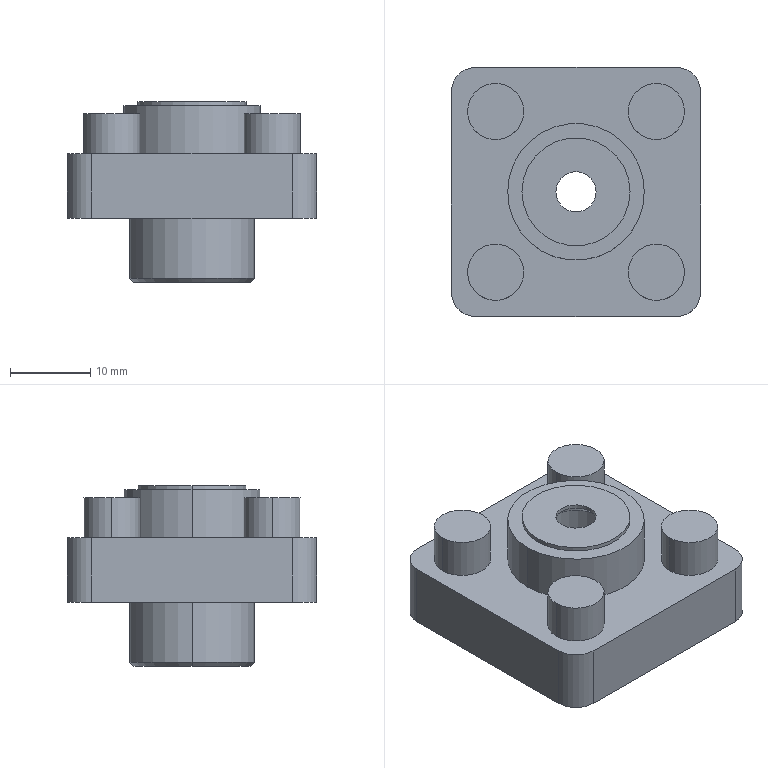Part | NX | features BREP 1 | 1 solid | 62 faces | box 31 x 31 x 22.5 mm | volume 8895 mm3 | cylinder 28 | plane 20 | cone 14 | commonest cylinder face diameters 7 x8 4 x4 6 x4 5 x2 9 x2 12 x2